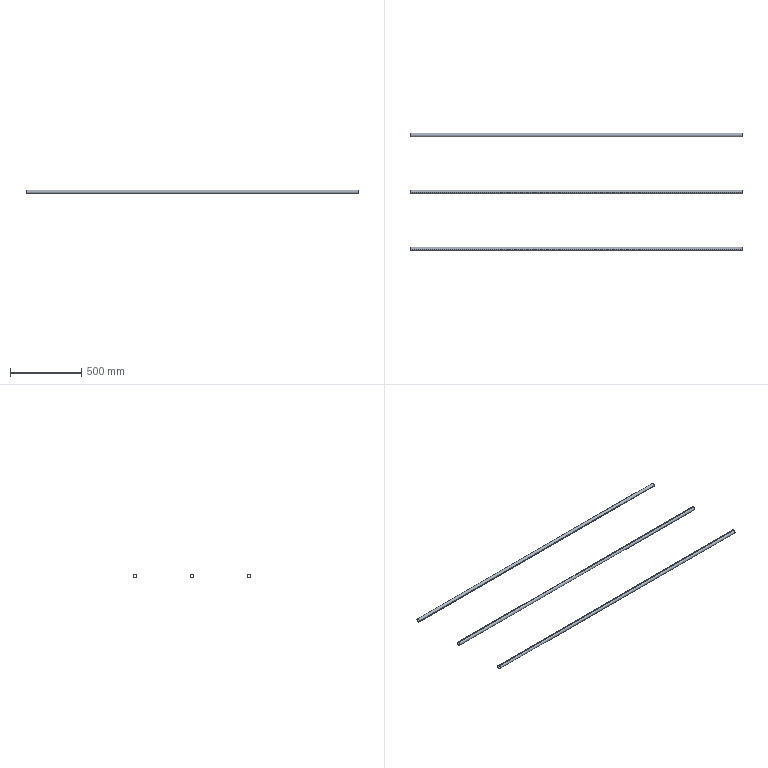Part | STEP file | 粉仓护栏栏杆9_Default<As Machined> | 3 solids | 18 faces | box 2325 x 825 x 25 mm | volume 772419 mm3 | cylinder 12 | plane 6 | commonest cylinder face diameters 22 x6 25 x6
STEP:
#1=CARTESIAN_POINT('',(0.,0.,0.));
#2=DIRECTION('',(0.,0.,1.));
#3=DIRECTION('',(1.,0.,0.));
#4=AXIS2_PLACEMENT_3D('',#1,#2,#3);
#5=CARTESIAN_POINT('',(-2325.,0.,12.5));
#6=VERTEX_POINT('',#5);
#7=CARTESIAN_POINT('',(-2325.,0.,-12.5));
#8=VERTEX_POINT('',#7);
#9=CARTESIAN_POINT('',(-2325.,0.,0.));
#10=DIRECTION('',(-1.,0.,0.));
#11=DIRECTION('',(0.,-1.,0.));
#12=AXIS2_PLACEMENT_3D('',#9,#10,#11);
#13=CIRCLE('',#12,12.5);
#14=CARTESIAN_POINT('',(-2325.,0.,0.));
#15=DIRECTION('',(1.,0.,0.));
#16=DIRECTION('',(0.,0.,-1.));
#17=AXIS2_PLACEMENT_3D('',#14,#15,#16);
#18=CYLINDRICAL_SURFACE('',#17,12.5);
#19=CARTESIAN_POINT('',(4.712,0.));
#20=DIRECTION('',(-1.,0.));
#21=VECTOR('',#20,1.);
#22=LINE('',#19,#21);
#23=(GEOMETRIC_REPRESENTATION_CONTEXT(2)PARAMETRIC_REPRESENTATION_CONTEXT()REPRESENTATION_CONTEXT('',''));
#24=DEFINITIONAL_REPRESENTATION('',(#22),#23);
#25=PCURVE('',#18,#24);
#26=CARTESIAN_POINT('',(-2325.,0.,0.));
#27=DIRECTION('',(-1.,0.,0.));
#28=DIRECTION('',(0.,-1.,0.));
#29=AXIS2_PLACEMENT_3D('',#26,#27,#28);
#30=PLANE('',#29);
#31=CARTESIAN_POINT('',(0.,0.));
#32=DIRECTION('',(1.,0.));
#33=AXIS2_PLACEMENT_2D('',#31,#32);
#34=CIRCLE('',#33,12.5);
#35=(GEOMETRIC_REPRESENTATION_CONTEXT(2)PARAMETRIC_REPRESENTATION_CONTEXT()REPRESENTATION_CONTEXT('',''));
#36=DEFINITIONAL_REPRESENTATION('',(#34),#35);
#37=PCURVE('',#30,#36);
#38=SURFACE_CURVE('',#13,(#25,#37),.PCURVE_S1.);
#39=EDGE_CURVE('',#6,#8,#38,.T.);
#40=ORIENTED_EDGE('',*,*,#39,.F.);
#41=CARTESIAN_POINT('',(0.,0.,12.5));
#42=VERTEX_POINT('',#41);
#43=CARTESIAN_POINT('',(-2325.,0.,12.5));
#44=DIRECTION('',(1.,0.,0.));
#45=VECTOR('',#44,1.);
#46=LINE('',#43,#45);
#47=CARTESIAN_POINT('',(3.142,0.));
#48=DIRECTION('',(0.,1.));
#49=VECTOR('',#48,1.);
#50=LINE('',#47,#49);
#51=(GEOMETRIC_REPRESENTATION_CONTEXT(2)PARAMETRIC_REPRESENTATION_CONTEXT()REPRESENTATION_CONTEXT('',''));
#52=DEFINITIONAL_REPRESENTATION('',(#50),#51);
#53=PCURVE('',#18,#52);
#54=CARTESIAN_POINT('',(-2325.,0.,0.));
#55=DIRECTION('',(1.,0.,0.));
#56=DIRECTION('',(0.,0.,-1.));
#57=AXIS2_PLACEMENT_3D('',#54,#55,#56);
#58=CYLINDRICAL_SURFACE('',#57,12.5);
#59=CARTESIAN_POINT('',(3.142,0.));
#60=DIRECTION('',(0.,1.));
#61=VECTOR('',#60,1.);
#62=LINE('',#59,#61);
#63=(GEOMETRIC_REPRESENTATION_CONTEXT(2)PARAMETRIC_REPRESENTATION_CONTEXT()REPRESENTATION_CONTEXT('',''));
#64=DEFINITIONAL_REPRESENTATION('',(#62),#63);
#65=PCURVE('',#58,#64);
#66=SURFACE_CURVE('',#46,(#53,#65),.PCURVE_S1.);
#67=EDGE_CURVE('',#6,#42,#66,.T.);
#68=ORIENTED_EDGE('',*,*,#67,.T.);
#69=CARTESIAN_POINT('',(0.,0.,-12.5));
#70=VERTEX_POINT('',#69);
#71=CARTESIAN_POINT('',(0.,0.,0.));
#72=DIRECTION('',(-1.,0.,0.));
#73=DIRECTION('',(0.,-1.,0.));
#74=AXIS2_PLACEMENT_3D('',#71,#72,#73);
#75=CIRCLE('',#74,12.5);
#76=CARTESIAN_POINT('',(4.712,2325.));
#77=DIRECTION('',(-1.,0.));
#78=VECTOR('',#77,1.);
#79=LINE('',#76,#78);
#80=(GEOMETRIC_REPRESENTATION_CONTEXT(2)PARAMETRIC_REPRESENTATION_CONTEXT()REPRESENTATION_CONTEXT('',''));
#81=DEFINITIONAL_REPRESENTATION('',(#79),#80);
#82=PCURVE('',#18,#81);
#83=CARTESIAN_POINT('',(0.,0.,0.));
#84=DIRECTION('',(-1.,0.,0.));
#85=DIRECTION('',(0.,-1.,0.));
#86=AXIS2_PLACEMENT_3D('',#83,#84,#85);
#87=PLANE('',#86);
#88=CARTESIAN_POINT('',(0.,0.));
#89=DIRECTION('',(1.,0.));
#90=AXIS2_PLACEMENT_2D('',#88,#89);
#91=CIRCLE('',#90,12.5);
#92=(GEOMETRIC_REPRESENTATION_CONTEXT(2)PARAMETRIC_REPRESENTATION_CONTEXT()REPRESENTATION_CONTEXT('',''));
#93=DEFINITIONAL_REPRESENTATION('',(#91),#92);
#94=PCURVE('',#87,#93);
#95=SURFACE_CURVE('',#75,(#82,#94),.PCURVE_S1.);
#96=EDGE_CURVE('',#42,#70,#95,.T.);
#97=ORIENTED_EDGE('',*,*,#96,.T.);
#98=CARTESIAN_POINT('',(-2325.,0.,-12.5));
#99=DIRECTION('',(1.,0.,0.));
#100=VECTOR('',#99,1.);
#101=LINE('',#98,#100);
#102=CARTESIAN_POINT('',(0.,0.));
#103=DIRECTION('',(0.,1.));
#104=VECTOR('',#103,1.);
#105=LINE('',#102,#104);
#106=(GEOMETRIC_REPRESENTATION_CONTEXT(2)PARAMETRIC_REPRESENTATION_CONTEXT()REPRESENTATION_CONTEXT('',''));
#107=DEFINITIONAL_REPRESENTATION('',(#105),#106);
#108=PCURVE('',#18,#107);
#109=CARTESIAN_POINT('',(6.283,0.));
#110=DIRECTION('',(0.,1.));
#111=VECTOR('',#110,1.);
#112=LINE('',#109,#111);
#113=(GEOMETRIC_REPRESENTATION_CONTEXT(2)PARAMETRIC_REPRESENTATION_CONTEXT()REPRESENTATION_CONTEXT('',''));
#114=DEFINITIONAL_REPRESENTATION('',(#112),#113);
#115=PCURVE('',#58,#114);
#116=SURFACE_CURVE('',#101,(#108,#115),.PCURVE_S1.);
#117=EDGE_CURVE('',#8,#70,#116,.T.);
#118=ORIENTED_EDGE('',*,*,#117,.F.);
#119=EDGE_LOOP('',(#40,#68,#97,#118));
#120=FACE_BOUND('',#119,.T.);
#121=ADVANCED_FACE('',(#120),#18,.T.);
#122=CARTESIAN_POINT('',(-2325.,0.,-11.));
#123=VERTEX_POINT('',#122);
#124=CARTESIAN_POINT('',(0.,0.,-11.));
#125=VERTEX_POINT('',#124);
#126=CARTESIAN_POINT('',(-2325.,0.,-11.));
#127=DIRECTION('',(1.,0.,0.));
#128=VECTOR('',#127,1.);
#129=LINE('',#126,#128);
#130=CARTESIAN_POINT('',(-2325.,0.,0.));
#131=DIRECTION('',(1.,0.,0.));
#132=DIRECTION('',(0.,0.,-1.));
#133=AXIS2_PLACEMENT_3D('',#130,#131,#132);
#134=CYLINDRICAL_SURFACE('',#133,11.);
#135=CARTESIAN_POINT('',(6.283,0.));
#136=DIRECTION('',(0.,1.));
#137=VECTOR('',#136,1.);
#138=LINE('',#135,#137);
#139=(GEOMETRIC_REPRESENTATION_CONTEXT(2)PARAMETRIC_REPRESENTATION_CONTEXT()REPRESENTATION_CONTEXT('',''));
#140=DEFINITIONAL_REPRESENTATION('',(#138),#139);
#141=PCURVE('',#134,#140);
#142=CARTESIAN_POINT('',(-2325.,0.,0.));
#143=DIRECTION('',(1.,0.,0.));
#144=DIRECTION('',(0.,0.,-1.));
#145=AXIS2_PLACEMENT_3D('',#142,#143,#144);
#146=CYLINDRICAL_SURFACE('',#145,11.);
#147=CARTESIAN_POINT('',(0.,0.));
#148=DIRECTION('',(0.,1.));
#149=VECTOR('',#148,1.);
#150=LINE('',#147,#149);
#151=(GEOMETRIC_REPRESENTATION_CONTEXT(2)PARAMETRIC_REPRESENTATION_CONTEXT()REPRESENTATION_CONTEXT('',''));
#152=DEFINITIONAL_REPRESENTATION('',(#150),#151);
#153=PCURVE('',#146,#152);
#154=SURFACE_CURVE('',#129,(#141,#153),.PCURVE_S1.);
#155=EDGE_CURVE('',#123,#125,#154,.T.);
#156=ORIENTED_EDGE('',*,*,#155,.T.);
#157=CARTESIAN_POINT('',(0.,0.,11.));
#158=VERTEX_POINT('',#157);
#159=CARTESIAN_POINT('',(0.,0.,0.));
#160=DIRECTION('',(-1.,0.,0.));
#161=DIRECTION('',(0.,-1.,0.));
#162=AXIS2_PLACEMENT_3D('',#159,#160,#161);
#163=CIRCLE('',#162,11.);
#164=CARTESIAN_POINT('',(10.996,2325.));
#165=DIRECTION('',(-1.,0.));
#166=VECTOR('',#165,1.);
#167=LINE('',#164,#166);
#168=(GEOMETRIC_REPRESENTATION_CONTEXT(2)PARAMETRIC_REPRESENTATION_CONTEXT()REPRESENTATION_CONTEXT('',''));
#169=DEFINITIONAL_REPRESENTATION('',(#167),#168);
#170=PCURVE('',#134,#169);
#171=CARTESIAN_POINT('',(0.,0.));
#172=DIRECTION('',(1.,0.));
#173=AXIS2_PLACEMENT_2D('',#171,#172);
#174=CIRCLE('',#173,11.);
#175=(GEOMETRIC_REPRESENTATION_CONTEXT(2)PARAMETRIC_REPRESENTATION_CONTEXT()REPRESENTATION_CONTEXT('',''));
#176=DEFINITIONAL_REPRESENTATION('',(#174),#175);
#177=PCURVE('',#87,#176);
#178=SURFACE_CURVE('',#163,(#170,#177),.PCURVE_S1.);
#179=EDGE_CURVE('',#125,#158,#178,.T.);
#180=ORIENTED_EDGE('',*,*,#179,.T.);
#181=CARTESIAN_POINT('',(-2325.,0.,11.));
#182=VERTEX_POINT('',#181);
#183=CARTESIAN_POINT('',(-2325.,0.,11.));
#184=DIRECTION('',(1.,0.,0.));
#185=VECTOR('',#184,1.);
#186=LINE('',#183,#185);
#187=CARTESIAN_POINT('',(3.142,0.));
#188=DIRECTION('',(0.,1.));
#189=VECTOR('',#188,1.);
#190=LINE('',#187,#189);
#191=(GEOMETRIC_REPRESENTATION_CONTEXT(2)PARAMETRIC_REPRESENTATION_CONTEXT()REPRESENTATION_CONTEXT('',''));
#192=DEFINITIONAL_REPRESENTATION('',(#190),#191);
#193=PCURVE('',#134,#192);
#194=CARTESIAN_POINT('',(3.142,0.));
#195=DIRECTION('',(0.,1.));
#196=VECTOR('',#195,1.);
#197=LINE('',#194,#196);
#198=(GEOMETRIC_REPRESENTATION_CONTEXT(2)PARAMETRIC_REPRESENTATION_CONTEXT()REPRESENTATION_CONTEXT('',''));
#199=DEFINITIONAL_REPRESENTATION('',(#197),#198);
#200=PCURVE('',#146,#199);
#201=SURFACE_CURVE('',#186,(#193,#200),.PCURVE_S1.);
#202=EDGE_CURVE('',#182,#158,#201,.T.);
#203=ORIENTED_EDGE('',*,*,#202,.F.);
#204=CARTESIAN_POINT('',(-2325.,0.,0.));
#205=DIRECTION('',(-1.,0.,0.));
#206=DIRECTION('',(0.,-1.,0.));
#207=AXIS2_PLACEMENT_3D('',#204,#205,#206);
#208=CIRCLE('',#207,11.);
#209=CARTESIAN_POINT('',(10.996,0.));
#210=DIRECTION('',(-1.,0.));
#211=VECTOR('',#210,1.);
#212=LINE('',#209,#211);
#213=(GEOMETRIC_REPRESENTATION_CONTEXT(2)PARAMETRIC_REPRESENTATION_CONTEXT()REPRESENTATION_CONTEXT('',''));
#214=DEFINITIONAL_REPRESENTATION('',(#212),#213);
#215=PCURVE('',#134,#214);
#216=CARTESIAN_POINT('',(0.,0.));
#217=DIRECTION('',(1.,0.));
#218=AXIS2_PLACEMENT_2D('',#216,#217);
#219=CIRCLE('',#218,11.);
#220=(GEOMETRIC_REPRESENTATION_CONTEXT(2)PARAMETRIC_REPRESENTATION_CONTEXT()REPRESENTATION_CONTEXT('',''));
#221=DEFINITIONAL_REPRESENTATION('',(#219),#220);
#222=PCURVE('',#30,#221);
#223=SURFACE_CURVE('',#208,(#215,#222),.PCURVE_S1.);
#224=EDGE_CURVE('',#123,#182,#223,.T.);
#225=ORIENTED_EDGE('',*,*,#224,.F.);
#226=EDGE_LOOP('',(#156,#180,#203,#225));
#227=FACE_BOUND('',#226,.F.);
#228=ADVANCED_FACE('',(#227),#134,.F.);
#229=CARTESIAN_POINT('',(0.,0.,0.));
#230=DIRECTION('',(-1.,0.,0.));
#231=DIRECTION('',(0.,-1.,0.));
#232=AXIS2_PLACEMENT_3D('',#229,#230,#231);
#233=CIRCLE('',#232,11.);
#234=CARTESIAN_POINT('',(4.712,2325.));
#235=DIRECTION('',(-1.,0.));
#236=VECTOR('',#235,1.);
#237=LINE('',#234,#236);
#238=(GEOMETRIC_REPRESENTATION_CONTEXT(2)PARAMETRIC_REPRESENTATION_CONTEXT()REPRESENTATION_CONTEXT('',''));
#239=DEFINITIONAL_REPRESENTATION('',(#237),#238);
#240=PCURVE('',#146,#239);
#241=CARTESIAN_POINT('',(0.,0.));
#242=DIRECTION('',(1.,0.));
#243=AXIS2_PLACEMENT_2D('',#241,#242);
#244=CIRCLE('',#243,11.);
#245=(GEOMETRIC_REPRESENTATION_CONTEXT(2)PARAMETRIC_REPRESENTATION_CONTEXT()REPRESENTATION_CONTEXT('',''));
#246=DEFINITIONAL_REPRESENTATION('',(#244),#245);
#247=PCURVE('',#87,#246);
#248=SURFACE_CURVE('',#233,(#240,#247),.PCURVE_S1.);
#249=EDGE_CURVE('',#158,#125,#248,.T.);
#250=ORIENTED_EDGE('',*,*,#249,.T.);
#251=ORIENTED_EDGE('',*,*,#155,.F.);
#252=CARTESIAN_POINT('',(-2325.,0.,0.));
#253=DIRECTION('',(-1.,0.,0.));
#254=DIRECTION('',(0.,-1.,0.));
#255=AXIS2_PLACEMENT_3D('',#252,#253,#254);
#256=CIRCLE('',#255,11.);
#257=CARTESIAN_POINT('',(4.712,0.));
#258=DIRECTION('',(-1.,0.));
#259=VECTOR('',#258,1.);
#260=LINE('',#257,#259);
#261=(GEOMETRIC_REPRESENTATION_CONTEXT(2)PARAMETRIC_REPRESENTATION_CONTEXT()REPRESENTATION_CONTEXT('',''));
#262=DEFINITIONAL_REPRESENTATION('',(#260),#261);
#263=PCURVE('',#146,#262);
#264=CARTESIAN_POINT('',(0.,0.));
#265=DIRECTION('',(1.,0.));
#266=AXIS2_PLACEMENT_2D('',#264,#265);
#267=CIRCLE('',#266,11.);
#268=(GEOMETRIC_REPRESENTATION_CONTEXT(2)PARAMETRIC_REPRESENTATION_CONTEXT()REPRESENTATION_CONTEXT('',''));
#269=DEFINITIONAL_REPRESENTATION('',(#267),#268);
#270=PCURVE('',#30,#269);
#271=SURFACE_CURVE('',#256,(#263,#270),.PCURVE_S1.);
#272=EDGE_CURVE('',#182,#123,#271,.T.);
#273=ORIENTED_EDGE('',*,*,#272,.F.);
#274=ORIENTED_EDGE('',*,*,#202,.T.);
#275=EDGE_LOOP('',(#250,#251,#273,#274));
#276=FACE_BOUND('',#275,.F.);
#277=ADVANCED_FACE('',(#276),#146,.F.);
#278=ORIENTED_EDGE('',*,*,#67,.F.);
#279=CARTESIAN_POINT('',(-2325.,0.,0.));
#280=DIRECTION('',(-1.,0.,0.));
#281=DIRECTION('',(0.,-1.,0.));
#282=AXIS2_PLACEMENT_3D('',#279,#280,#281);
#283=CIRCLE('',#282,12.5);
#284=CARTESIAN_POINT('',(10.996,0.));
#285=DIRECTION('',(-1.,0.));
#286=VECTOR('',#285,1.);
#287=LINE('',#284,#286);
#288=(GEOMETRIC_REPRESENTATION_CONTEXT(2)PARAMETRIC_REPRESENTATION_CONTEXT()REPRESENTATION_CONTEXT('',''));
#289=DEFINITIONAL_REPRESENTATION('',(#287),#288);
#290=PCURVE('',#58,#289);
#291=CARTESIAN_POINT('',(0.,0.));
#292=DIRECTION('',(1.,0.));
#293=AXIS2_PLACEMENT_2D('',#291,#292);
#294=CIRCLE('',#293,12.5);
#295=(GEOMETRIC_REPRESENTATION_CONTEXT(2)PARAMETRIC_REPRESENTATION_CONTEXT()REPRESENTATION_CONTEXT('',''));
#296=DEFINITIONAL_REPRESENTATION('',(#294),#295);
#297=PCURVE('',#30,#296);
#298=SURFACE_CURVE('',#283,(#290,#297),.PCURVE_S1.);
#299=EDGE_CURVE('',#8,#6,#298,.T.);
#300=ORIENTED_EDGE('',*,*,#299,.F.);
#301=ORIENTED_EDGE('',*,*,#117,.T.);
#302=CARTESIAN_POINT('',(0.,0.,0.));
#303=DIRECTION('',(-1.,0.,0.));
#304=DIRECTION('',(0.,-1.,0.));
#305=AXIS2_PLACEMENT_3D('',#302,#303,#304);
#306=CIRCLE('',#305,12.5);
#307=CARTESIAN_POINT('',(10.996,2325.));
#308=DIRECTION('',(-1.,0.));
#309=VECTOR('',#308,1.);
#310=LINE('',#307,#309);
#311=(GEOMETRIC_REPRESENTATION_CONTEXT(2)PARAMETRIC_REPRESENTATION_CONTEXT()REPRESENTATION_CONTEXT('',''));
#312=DEFINITIONAL_REPRESENTATION('',(#310),#311);
#313=PCURVE('',#58,#312);
#314=CARTESIAN_POINT('',(0.,0.));
#315=DIRECTION('',(1.,0.));
#316=AXIS2_PLACEMENT_2D('',#314,#315);
#317=CIRCLE('',#316,12.5);
#318=(GEOMETRIC_REPRESENTATION_CONTEXT(2)PARAMETRIC_REPRESENTATION_CONTEXT()REPRESENTATION_CONTEXT('',''));
#319=DEFINITIONAL_REPRESENTATION('',(#317),#318);
#320=PCURVE('',#87,#319);
#321=SURFACE_CURVE('',#306,(#313,#320),.PCURVE_S1.);
#322=EDGE_CURVE('',#70,#42,#321,.T.);
#323=ORIENTED_EDGE('',*,*,#322,.T.);
#324=EDGE_LOOP('',(#278,#300,#301,#323));
#325=FACE_BOUND('',#324,.T.);
#326=ADVANCED_FACE('',(#325),#58,.T.);
#327=ORIENTED_EDGE('',*,*,#224,.F.);
#328=ORIENTED_EDGE('',*,*,#272,.F.);
#329=EDGE_LOOP('',(#327,#328));
#330=FACE_BOUND('',#329,.T.);
#331=ORIENTED_EDGE('',*,*,#299,.T.);
#332=ORIENTED_EDGE('',*,*,#39,.T.);
#333=EDGE_LOOP('',(#331,#332));
#334=FACE_BOUND('',#333,.T.);
#335=ADVANCED_FACE('',(#330,#334),#30,.T.);
#336=ORIENTED_EDGE('',*,*,#179,.T.);
#337=ORIENTED_EDGE('',*,*,#249,.T.);
#338=EDGE_LOOP('',(#336,#337));
#339=FACE_BOUND('',#338,.T.);
#340=ORIENTED_EDGE('',*,*,#322,.F.);
#341=ORIENTED_EDGE('',*,*,#96,.F.);
#342=EDGE_LOOP('',(#340,#341));
#343=FACE_BOUND('',#342,.T.);
#344=ADVANCED_FACE('',(#339,#343),#87,.F.);
#345=CLOSED_SHELL('',(#121,#228,#277,#326,#335,#344));
#346=MANIFOLD_SOLID_BREP('',#345);
#347=CARTESIAN_POINT('',(-2325.,787.5,0.));
#348=VERTEX_POINT('',#347);
#349=CARTESIAN_POINT('',(-2325.,812.5,0.));
#350=VERTEX_POINT('',#349);
#351=CARTESIAN_POINT('',(-2325.,800.,0.));
#352=DIRECTION('',(-1.,0.,0.));
#353=DIRECTION('',(0.,-1.,0.));
#354=AXIS2_PLACEMENT_3D('',#351,#352,#353);
#355=CIRCLE('',#354,12.5);
#356=CARTESIAN_POINT('',(-2325.,800.,0.));
#357=DIRECTION('',(1.,0.,0.));
#358=DIRECTION('',(0.,1.,0.));
#359=AXIS2_PLACEMENT_3D('',#356,#357,#358);
#360=CYLINDRICAL_SURFACE('',#359,12.5);
#361=CARTESIAN_POINT('',(3.142,0.));
#362=DIRECTION('',(-1.,0.));
#363=VECTOR('',#362,1.);
#364=LINE('',#361,#363);
#365=(GEOMETRIC_REPRESENTATION_CONTEXT(2)PARAMETRIC_REPRESENTATION_CONTEXT()REPRESENTATION_CONTEXT('',''));
#366=DEFINITIONAL_REPRESENTATION('',(#364),#365);
#367=PCURVE('',#360,#366);
#368=CARTESIAN_POINT('',(-2325.,800.,0.));
#369=DIRECTION('',(-1.,0.,0.));
#370=DIRECTION('',(0.,-1.,0.));
#371=AXIS2_PLACEMENT_3D('',#368,#369,#370);
#372=PLANE('',#371);
#373=CARTESIAN_POINT('',(0.,0.));
#374=DIRECTION('',(1.,0.));
#375=AXIS2_PLACEMENT_2D('',#373,#374);
#376=CIRCLE('',#375,12.5);
#377=(GEOMETRIC_REPRESENTATION_CONTEXT(2)PARAMETRIC_REPRESENTATION_CONTEXT()REPRESENTATION_CONTEXT('',''));
#378=DEFINITIONAL_REPRESENTATION('',(#376),#377);
#379=PCURVE('',#372,#378);
#380=SURFACE_CURVE('',#355,(#367,#379),.PCURVE_S1.);
#381=EDGE_CURVE('',#348,#350,#380,.T.);
#382=ORIENTED_EDGE('',*,*,#381,.F.);
#383=CARTESIAN_POINT('',(0.,787.5,0.));
#384=VERTEX_POINT('',#383);
#385=CARTESIAN_POINT('',(-2325.,787.5,0.));
#386=DIRECTION('',(1.,0.,0.));
#387=VECTOR('',#386,1.);
#388=LINE('',#385,#387);
#389=CARTESIAN_POINT('',(3.142,0.));
#390=DIRECTION('',(0.,1.));
#391=VECTOR('',#390,1.);
#392=LINE('',#389,#391);
#393=(GEOMETRIC_REPRESENTATION_CONTEXT(2)PARAMETRIC_REPRESENTATION_CONTEXT()REPRESENTATION_CONTEXT('',''));
#394=DEFINITIONAL_REPRESENTATION('',(#392),#393);
#395=PCURVE('',#360,#394);
#396=CARTESIAN_POINT('',(-2325.,800.,0.));
#397=DIRECTION('',(1.,0.,0.));
#398=DIRECTION('',(0.,1.,0.));
#399=AXIS2_PLACEMENT_3D('',#396,#397,#398);
#400=CYLINDRICAL_SURFACE('',#399,12.5);
#401=CARTESIAN_POINT('',(3.142,0.));
#402=DIRECTION('',(0.,1.));
#403=VECTOR('',#402,1.);
#404=LINE('',#401,#403);
#405=(GEOMETRIC_REPRESENTATION_CONTEXT(2)PARAMETRIC_REPRESENTATION_CONTEXT()REPRESENTATION_CONTEXT('',''));
#406=DEFINITIONAL_REPRESENTATION('',(#404),#405);
#407=PCURVE('',#400,#406);
#408=SURFACE_CURVE('',#388,(#395,#407),.PCURVE_S1.);
#409=EDGE_CURVE('',#348,#384,#408,.T.);
#410=ORIENTED_EDGE('',*,*,#409,.T.);
#411=CARTESIAN_POINT('',(0.,812.5,0.));
#412=VERTEX_POINT('',#411);
#413=CARTESIAN_POINT('',(0.,800.,0.));
#414=DIRECTION('',(-1.,0.,0.));
#415=DIRECTION('',(0.,-1.,0.));
#416=AXIS2_PLACEMENT_3D('',#413,#414,#415);
#417=CIRCLE('',#416,12.5);
#418=CARTESIAN_POINT('',(3.142,2325.));
#419=DIRECTION('',(-1.,0.));
#420=VECTOR('',#419,1.);
#421=LINE('',#418,#420);
#422=(GEOMETRIC_REPRESENTATION_CONTEXT(2)PARAMETRIC_REPRESENTATION_CONTEXT()REPRESENTATION_CONTEXT('',''));
#423=DEFINITIONAL_REPRESENTATION('',(#421),#422);
#424=PCURVE('',#360,#423);
#425=CARTESIAN_POINT('',(0.,800.,0.));
#426=DIRECTION('',(-1.,0.,0.));
#427=DIRECTION('',(0.,-1.,0.));
#428=AXIS2_PLACEMENT_3D('',#425,#426,#427);
#429=PLANE('',#428);
#430=CARTESIAN_POINT('',(0.,0.));
#431=DIRECTION('',(1.,0.));
#432=AXIS2_PLACEMENT_2D('',#430,#431);
#433=CIRCLE('',#432,12.5);
#434=(GEOMETRIC_REPRESENTATION_CONTEXT(2)PARAMETRIC_REPRESENTATION_CONTEXT()REPRESENTATION_CONTEXT('',''));
#435=DEFINITIONAL_REPRESENTATION('',(#433),#434);
#436=PCURVE('',#429,#435);
#437=SURFACE_CURVE('',#417,(#424,#436),.PCURVE_S1.);
#438=EDGE_CURVE('',#384,#412,#437,.T.);
#439=ORIENTED_EDGE('',*,*,#438,.T.);
#440=CARTESIAN_POINT('',(-2325.,812.5,0.));
#441=DIRECTION('',(1.,0.,0.));
#442=VECTOR('',#441,1.);
#443=LINE('',#440,#442);
#444=CARTESIAN_POINT('',(0.,0.));
#445=DIRECTION('',(0.,1.));
#446=VECTOR('',#445,1.);
#447=LINE('',#444,#446);
#448=(GEOMETRIC_REPRESENTATION_CONTEXT(2)PARAMETRIC_REPRESENTATION_CONTEXT()REPRESENTATION_CONTEXT('',''));
#449=DEFINITIONAL_REPRESENTATION('',(#447),#448);
#450=PCURVE('',#360,#449);
#451=CARTESIAN_POINT('',(6.283,0.));
#452=DIRECTION('',(0.,1.));
#453=VECTOR('',#452,1.);
#454=LINE('',#451,#453);
#455=(GEOMETRIC_REPRESENTATION_CONTEXT(2)PARAMETRIC_REPRESENTATION_CONTEXT()REPRESENTATION_CONTEXT('',''));
#456=DEFINITIONAL_REPRESENTATION('',(#454),#455);
#457=PCURVE('',#400,#456);
#458=SURFACE_CURVE('',#443,(#450,#457),.PCURVE_S1.);
#459=EDGE_CURVE('',#350,#412,#458,.T.);
#460=ORIENTED_EDGE('',*,*,#459,.F.);
#461=EDGE_LOOP('',(#382,#410,#439,#460));
#462=FACE_BOUND('',#461,.T.);
#463=ADVANCED_FACE('',(#462),#360,.T.);
#464=CARTESIAN_POINT('',(-2325.,811.,0.));
#465=VERTEX_POINT('',#464);
#466=CARTESIAN_POINT('',(0.,811.,0.));
#467=VERTEX_POINT('',#466);
#468=CARTESIAN_POINT('',(-2325.,811.,0.));
#469=DIRECTION('',(1.,0.,0.));
#470=VECTOR('',#469,1.);
#471=LINE('',#468,#470);
#472=CARTESIAN_POINT('',(-2325.,800.,0.));
#473=DIRECTION('',(1.,0.,0.));
#474=DIRECTION('',(0.,1.,0.));
#475=AXIS2_PLACEMENT_3D('',#472,#473,#474);
#476=CYLINDRICAL_SURFACE('',#475,11.);
#477=CARTESIAN_POINT('',(6.283,0.));
#478=DIRECTION('',(0.,1.));
#479=VECTOR('',#478,1.);
#480=LINE('',#477,#479);
#481=(GEOMETRIC_REPRESENTATION_CONTEXT(2)PARAMETRIC_REPRESENTATION_CONTEXT()REPRESENTATION_CONTEXT('',''));
#482=DEFINITIONAL_REPRESENTATION('',(#480),#481);
#483=PCURVE('',#476,#482);
#484=CARTESIAN_POINT('',(-2325.,800.,0.));
#485=DIRECTION('',(1.,0.,0.));
#486=DIRECTION('',(0.,1.,0.));
#487=AXIS2_PLACEMENT_3D('',#484,#485,#486);
#488=CYLINDRICAL_SURFACE('',#487,11.);
#489=CARTESIAN_POINT('',(0.,0.));
#490=DIRECTION('',(0.,1.));
#491=VECTOR('',#490,1.);
#492=LINE('',#489,#491);
#493=(GEOMETRIC_REPRESENTATION_CONTEXT(2)PARAMETRIC_REPRESENTATION_CONTEXT()REPRESENTATION_CONTEXT('',''));
#494=DEFINITIONAL_REPRESENTATION('',(#492),#493);
#495=PCURVE('',#488,#494);
#496=SURFACE_CURVE('',#471,(#483,#495),.PCURVE_S1.);
#497=EDGE_CURVE('',#465,#467,#496,.T.);
#498=ORIENTED_EDGE('',*,*,#497,.T.);
#499=CARTESIAN_POINT('',(0.,789.,0.));
#500=VERTEX_POINT('',#499);
#501=CARTESIAN_POINT('',(0.,800.,0.));
#502=DIRECTION('',(-1.,0.,0.));
#503=DIRECTION('',(0.,-1.,0.));
#504=AXIS2_PLACEMENT_3D('',#501,#502,#503);
#505=CIRCLE('',#504,11.);
#506=CARTESIAN_POINT('',(9.425,2325.));
#507=DIRECTION('',(-1.,0.));
#508=VECTOR('',#507,1.);
#509=LINE('',#506,#508);
#510=(GEOMETRIC_REPRESENTATION_CONTEXT(2)PARAMETRIC_REPRESENTATION_CONTEXT()REPRESENTATION_CONTEXT('',''));
#511=DEFINITIONAL_REPRESENTATION('',(#509),#510);
#512=PCURVE('',#476,#511);
#513=CARTESIAN_POINT('',(0.,0.));
#514=DIRECTION('',(1.,0.));
#515=AXIS2_PLACEMENT_2D('',#513,#514);
#516=CIRCLE('',#515,11.);
#517=(GEOMETRIC_REPRESENTATION_CONTEXT(2)PARAMETRIC_REPRESENTATION_CONTEXT()REPRESENTATION_CONTEXT('',''));
#518=DEFINITIONAL_REPRESENTATION('',(#516),#517);
#519=PCURVE('',#429,#518);
#520=SURFACE_CURVE('',#505,(#512,#519),.PCURVE_S1.);
#521=EDGE_CURVE('',#467,#500,#520,.T.);
#522=ORIENTED_EDGE('',*,*,#521,.T.);
#523=CARTESIAN_POINT('',(-2325.,789.,0.));
#524=VERTEX_POINT('',#523);
#525=CARTESIAN_POINT('',(-2325.,789.,0.));
#526=DIRECTION('',(1.,0.,0.));
#527=VECTOR('',#526,1.);
#528=LINE('',#525,#527);
#529=CARTESIAN_POINT('',(3.142,0.));
#530=DIRECTION('',(0.,1.));
#531=VECTOR('',#530,1.);
#532=LINE('',#529,#531);
#533=(GEOMETRIC_REPRESENTATION_CONTEXT(2)PARAMETRIC_REPRESENTATION_CONTEXT()REPRESENTATION_CONTEXT('',''));
#534=DEFINITIONAL_REPRESENTATION('',(#532),#533);
#535=PCURVE('',#476,#534);
#536=CARTESIAN_POINT('',(3.142,0.));
#537=DIRECTION('',(0.,1.));
#538=VECTOR('',#537,1.);
#539=LINE('',#536,#538);
#540=(GEOMETRIC_REPRESENTATION_CONTEXT(2)PARAMETRIC_REPRESENTATION_CONTEXT()REPRESENTATION_CONTEXT('',''));
#541=DEFINITIONAL_REPRESENTATION('',(#539),#540);
#542=PCURVE('',#488,#541);
#543=SURFACE_CURVE('',#528,(#535,#542),.PCURVE_S1.);
#544=EDGE_CURVE('',#524,#500,#543,.T.);
#545=ORIENTED_EDGE('',*,*,#544,.F.);
#546=CARTESIAN_POINT('',(-2325.,800.,0.));
#547=DIRECTION('',(-1.,0.,0.));
#548=DIRECTION('',(0.,-1.,0.));
#549=AXIS2_PLACEMENT_3D('',#546,#547,#548);
#550=CIRCLE('',#549,11.);
#551=CARTESIAN_POINT('',(9.425,0.));
#552=DIRECTION('',(-1.,0.));
#553=VECTOR('',#552,1.);
#554=LINE('',#551,#553);
#555=(GEOMETRIC_REPRESENTATION_CONTEXT(2)PARAMETRIC_REPRESENTATION_CONTEXT()REPRESENTATION_CONTEXT('',''));
#556=DEFINITIONAL_REPRESENTATION('',(#554),#555);
#557=PCURVE('',#476,#556);
#558=CARTESIAN_POINT('',(0.,0.));
#559=DIRECTION('',(1.,0.));
#560=AXIS2_PLACEMENT_2D('',#558,#559);
#561=CIRCLE('',#560,11.);
#562=(GEOMETRIC_REPRESENTATION_CONTEXT(2)PARAMETRIC_REPRESENTATION_CONTEXT()REPRESENTATION_CONTEXT('',''));
#563=DEFINITIONAL_REPRESENTATION('',(#561),#562);
#564=PCURVE('',#372,#563);
#565=SURFACE_CURVE('',#550,(#557,#564),.PCURVE_S1.);
#566=EDGE_CURVE('',#465,#524,#565,.T.);
#567=ORIENTED_EDGE('',*,*,#566,.F.);
#568=EDGE_LOOP('',(#498,#522,#545,#567));
#569=FACE_BOUND('',#568,.F.);
#570=ADVANCED_FACE('',(#569),#476,.F.);
#571=CARTESIAN_POINT('',(0.,800.,0.));
#572=DIRECTION('',(-1.,0.,0.));
#573=DIRECTION('',(0.,-1.,0.));
#574=AXIS2_PLACEMENT_3D('',#571,#572,#573);
#575=CIRCLE('',#574,11.);
#576=CARTESIAN_POINT('',(3.142,2325.));
#577=DIRECTION('',(-1.,0.));
#578=VECTOR('',#577,1.);
#579=LINE('',#576,#578);
#580=(GEOMETRIC_REPRESENTATION_CONTEXT(2)PARAMETRIC_REPRESENTATION_CONTEXT()REPRESENTATION_CONTEXT('',''));
#581=DEFINITIONAL_REPRESENTATION('',(#579),#580);
#582=PCURVE('',#488,#581);
#583=CARTESIAN_POINT('',(0.,0.));
#584=DIRECTION('',(1.,0.));
#585=AXIS2_PLACEMENT_2D('',#583,#584);
#586=CIRCLE('',#585,11.);
#587=(GEOMETRIC_REPRESENTATION_CONTEXT(2)PARAMETRIC_REPRESENTATION_CONTEXT()REPRESENTATION_CONTEXT('',''));
#588=DEFINITIONAL_REPRESENTATION('',(#586),#587);
#589=PCURVE('',#429,#588);
#590=SURFACE_CURVE('',#575,(#582,#589),.PCURVE_S1.);
#591=EDGE_CURVE('',#500,#467,#590,.T.);
#592=ORIENTED_EDGE('',*,*,#591,.T.);
#593=ORIENTED_EDGE('',*,*,#497,.F.);
#594=CARTESIAN_POINT('',(-2325.,800.,0.));
#595=DIRECTION('',(-1.,0.,0.));
#596=DIRECTION('',(0.,-1.,0.));
#597=AXIS2_PLACEMENT_3D('',#594,#595,#596);
#598=CIRCLE('',#597,11.);
#599=CARTESIAN_POINT('',(3.142,0.));
#600=DIRECTION('',(-1.,0.));
#601=VECTOR('',#600,1.);
#602=LINE('',#599,#601);
#603=(GEOMETRIC_REPRESENTATION_CONTEXT(2)PARAMETRIC_REPRESENTATION_CONTEXT()REPRESENTATION_CONTEXT('',''));
#604=DEFINITIONAL_REPRESENTATION('',(#602),#603);
#605=PCURVE('',#488,#604);
#606=CARTESIAN_POINT('',(0.,0.));
#607=DIRECTION('',(1.,0.));
#608=AXIS2_PLACEMENT_2D('',#606,#607);
#609=CIRCLE('',#608,11.);
#610=(GEOMETRIC_REPRESENTATION_CONTEXT(2)PARAMETRIC_REPRESENTATION_CONTEXT()REPRESENTATION_CONTEXT('',''));
#611=DEFINITIONAL_REPRESENTATION('',(#609),#610);
#612=PCURVE('',#372,#611);
#613=SURFACE_CURVE('',#598,(#605,#612),.PCURVE_S1.);
#614=EDGE_CURVE('',#524,#465,#613,.T.);
#615=ORIENTED_EDGE('',*,*,#614,.F.);
#616=ORIENTED_EDGE('',*,*,#544,.T.);
#617=EDGE_LOOP('',(#592,#593,#615,#616));
#618=FACE_BOUND('',#617,.F.);
#619=ADVANCED_FACE('',(#618),#488,.F.);
#620=ORIENTED_EDGE('',*,*,#409,.F.);
#621=CARTESIAN_POINT('',(-2325.,800.,0.));
#622=DIRECTION('',(-1.,0.,0.));
#623=DIRECTION('',(0.,-1.,0.));
#624=AXIS2_PLACEMENT_3D('',#621,#622,#623);
#625=CIRCLE('',#624,12.5);
#626=CARTESIAN_POINT('',(9.425,0.));
#627=DIRECTION('',(-1.,0.));
#628=VECTOR('',#627,1.);
#629=LINE('',#626,#628);
#630=(GEOMETRIC_REPRESENTATION_CONTEXT(2)PARAMETRIC_REPRESENTATION_CONTEXT()REPRESENTATION_CONTEXT('',''));
#631=DEFINITIONAL_REPRESENTATION('',(#629),#630);
#632=PCURVE('',#400,#631);
#633=CARTESIAN_POINT('',(0.,0.));
#634=DIRECTION('',(1.,0.));
#635=AXIS2_PLACEMENT_2D('',#633,#634);
#636=CIRCLE('',#635,12.5);
#637=(GEOMETRIC_REPRESENTATION_CONTEXT(2)PARAMETRIC_REPRESENTATION_CONTEXT()REPRESENTATION_CONTEXT('',''));
#638=DEFINITIONAL_REPRESENTATION('',(#636),#637);
#639=PCURVE('',#372,#638);
#640=SURFACE_CURVE('',#625,(#632,#639),.PCURVE_S1.);
#641=EDGE_CURVE('',#350,#348,#640,.T.);
#642=ORIENTED_EDGE('',*,*,#641,.F.);
#643=ORIENTED_EDGE('',*,*,#459,.T.);
#644=CARTESIAN_POINT('',(0.,800.,0.));
#645=DIRECTION('',(-1.,0.,0.));
#646=DIRECTION('',(0.,-1.,0.));
#647=AXIS2_PLACEMENT_3D('',#644,#645,#646);
#648=CIRCLE('',#647,12.5);
#649=CARTESIAN_POINT('',(9.425,2325.));
#650=DIRECTION('',(-1.,0.));
#651=VECTOR('',#650,1.);
#652=LINE('',#649,#651);
#653=(GEOMETRIC_REPRESENTATION_CONTEXT(2)PARAMETRIC_REPRESENTATION_CONTEXT()REPRESENTATION_CONTEXT('',''));
#654=DEFINITIONAL_REPRESENTATION('',(#652),#653);
#655=PCURVE('',#400,#654);
#656=CARTESIAN_POINT('',(0.,0.));
#657=DIRECTION('',(1.,0.));
#658=AXIS2_PLACEMENT_2D('',#656,#657);
#659=CIRCLE('',#658,12.5);
#660=(GEOMETRIC_REPRESENTATION_CONTEXT(2)PARAMETRIC_REPRESENTATION_CONTEXT()REPRESENTATION_CONTEXT('',''));
#661=DEFINITIONAL_REPRESENTATION('',(#659),#660);
#662=PCURVE('',#429,#661);
#663=SURFACE_CURVE('',#648,(#655,#662),.PCURVE_S1.);
#664=EDGE_CURVE('',#412,#384,#663,.T.);
#665=ORIENTED_EDGE('',*,*,#664,.T.);
#666=EDGE_LOOP('',(#620,#642,#643,#665));
#667=FACE_BOUND('',#666,.T.);
#668=ADVANCED_FACE('',(#667),#400,.T.);
#669=ORIENTED_EDGE('',*,*,#566,.F.);
#670=ORIENTED_EDGE('',*,*,#614,.F.);
#671=EDGE_LOOP('',(#669,#670));
#672=FACE_BOUND('',#671,.T.);
#673=ORIENTED_EDGE('',*,*,#641,.T.);
#674=ORIENTED_EDGE('',*,*,#381,.T.);
#675=EDGE_LOOP('',(#673,#674));
#676=FACE_BOUND('',#675,.T.);
#677=ADVANCED_FACE('',(#672,#676),#372,.T.);
#678=ORIENTED_EDGE('',*,*,#521,.T.);
#679=ORIENTED_EDGE('',*,*,#591,.T.);
#680=EDGE_LOOP('',(#678,#679));
#681=FACE_BOUND('',#680,.T.);
#682=ORIENTED_EDGE('',*,*,#664,.F.);
#683=ORIENTED_EDGE('',*,*,#438,.F.);
#684=EDGE_LOOP('',(#682,#683));
#685=FACE_BOUND('',#684,.T.);
#686=ADVANCED_FACE('',(#681,#685),#429,.F.);
#687=CLOSED_SHELL('',(#463,#570,#619,#668,#677,#686));
#688=MANIFOLD_SOLID_BREP('',#687);
#689=CARTESIAN_POINT('',(0.,400.,-12.5));
#690=VERTEX_POINT('',#689);
#691=CARTESIAN_POINT('',(0.,400.,12.5));
#692=VERTEX_POINT('',#691);
#693=CARTESIAN_POINT('',(0.,400.,0.));
#694=DIRECTION('',(1.,0.,0.));
#695=DIRECTION('',(0.,1.,0.));
#696=AXIS2_PLACEMENT_3D('',#693,#694,#695);
#697=CIRCLE('',#696,12.5);
#698=CARTESIAN_POINT('',(0.,400.,0.));
#699=DIRECTION('',(-1.,0.,0.));
#700=DIRECTION('',(0.,0.,1.));
#701=AXIS2_PLACEMENT_3D('',#698,#699,#700);
#702=CYLINDRICAL_SURFACE('',#701,12.5);
#703=CARTESIAN_POINT('',(7.854,0.));
#704=DIRECTION('',(-1.,0.));
#705=VECTOR('',#704,1.);
#706=LINE('',#703,#705);
#707=(GEOMETRIC_REPRESENTATION_CONTEXT(2)PARAMETRIC_REPRESENTATION_CONTEXT()REPRESENTATION_CONTEXT('',''));
#708=DEFINITIONAL_REPRESENTATION('',(#706),#707);
#709=PCURVE('',#702,#708);
#710=CARTESIAN_POINT('',(0.,400.,0.));
#711=DIRECTION('',(1.,0.,0.));
#712=DIRECTION('',(0.,1.,0.));
#713=AXIS2_PLACEMENT_3D('',#710,#711,#712);
#714=PLANE('',#713);
#715=CARTESIAN_POINT('',(0.,0.));
#716=DIRECTION('',(1.,0.));
#717=AXIS2_PLACEMENT_2D('',#715,#716);
#718=CIRCLE('',#717,12.5);
#719=(GEOMETRIC_REPRESENTATION_CONTEXT(2)PARAMETRIC_REPRESENTATION_CONTEXT()REPRESENTATION_CONTEXT('',''));
#720=DEFINITIONAL_REPRESENTATION('',(#718),#719);
#721=PCURVE('',#714,#720);
#722=SURFACE_CURVE('',#697,(#709,#721),.PCURVE_S1.);
#723=EDGE_CURVE('',#690,#692,#722,.T.);
#724=ORIENTED_EDGE('',*,*,#723,.F.);
#725=CARTESIAN_POINT('',(-2325.,400.,-12.5));
#726=VERTEX_POINT('',#725);
#727=CARTESIAN_POINT('',(0.,400.,-12.5));
#728=DIRECTION('',(-1.,0.,0.));
#729=VECTOR('',#728,1.);
#730=LINE('',#727,#729);
#731=CARTESIAN_POINT('',(3.142,0.));
#732=DIRECTION('',(0.,1.));
#733=VECTOR('',#732,1.);
#734=LINE('',#731,#733);
#735=(GEOMETRIC_REPRESENTATION_CONTEXT(2)PARAMETRIC_REPRESENTATION_CONTEXT()REPRESENTATION_CONTEXT('',''));
#736=DEFINITIONAL_REPRESENTATION('',(#734),#735);
#737=PCURVE('',#702,#736);
#738=CARTESIAN_POINT('',(0.,400.,0.));
#739=DIRECTION('',(-1.,0.,0.));
#740=DIRECTION('',(0.,0.,1.));
#741=AXIS2_PLACEMENT_3D('',#738,#739,#740);
#742=CYLINDRICAL_SURFACE('',#741,12.5);
#743=CARTESIAN_POINT('',(3.142,0.));
#744=DIRECTION('',(0.,1.));
#745=VECTOR('',#744,1.);
#746=LINE('',#743,#745);
#747=(GEOMETRIC_REPRESENTATION_CONTEXT(2)PARAMETRIC_REPRESENTATION_CONTEXT()REPRESENTATION_CONTEXT('',''));
#748=DEFINITIONAL_REPRESENTATION('',(#746),#747);
#749=PCURVE('',#742,#748);
#750=SURFACE_CURVE('',#730,(#737,#749),.PCURVE_S1.);
#751=EDGE_CURVE('',#690,#726,#750,.T.);
#752=ORIENTED_EDGE('',*,*,#751,.T.);
#753=CARTESIAN_POINT('',(-2325.,400.,12.5));
#754=VERTEX_POINT('',#753);
#755=CARTESIAN_POINT('',(-2325.,400.,0.));
#756=DIRECTION('',(1.,0.,0.));
#757=DIRECTION('',(0.,1.,0.));
#758=AXIS2_PLACEMENT_3D('',#755,#756,#757);
#759=CIRCLE('',#758,12.5);
#760=CARTESIAN_POINT('',(7.854,2325.));
#761=DIRECTION('',(-1.,0.));
#762=VECTOR('',#761,1.);
#763=LINE('',#760,#762);
#764=(GEOMETRIC_REPRESENTATION_CONTEXT(2)PARAMETRIC_REPRESENTATION_CONTEXT()REPRESENTATION_CONTEXT('',''));
#765=DEFINITIONAL_REPRESENTATION('',(#763),#764);
#766=PCURVE('',#702,#765);
#767=CARTESIAN_POINT('',(-2325.,400.,0.));
#768=DIRECTION('',(1.,0.,0.));
#769=DIRECTION('',(0.,1.,0.));
#770=AXIS2_PLACEMENT_3D('',#767,#768,#769);
#771=PLANE('',#770);
#772=CARTESIAN_POINT('',(0.,0.));
#773=DIRECTION('',(1.,0.));
#774=AXIS2_PLACEMENT_2D('',#772,#773);
#775=CIRCLE('',#774,12.5);
#776=(GEOMETRIC_REPRESENTATION_CONTEXT(2)PARAMETRIC_REPRESENTATION_CONTEXT()REPRESENTATION_CONTEXT('',''));
#777=DEFINITIONAL_REPRESENTATION('',(#775),#776);
#778=PCURVE('',#771,#777);
#779=SURFACE_CURVE('',#759,(#766,#778),.PCURVE_S1.);
#780=EDGE_CURVE('',#726,#754,#779,.T.);
#781=ORIENTED_EDGE('',*,*,#780,.T.);
#782=CARTESIAN_POINT('',(0.,400.,12.5));
#783=DIRECTION('',(-1.,0.,0.));
#784=VECTOR('',#783,1.);
#785=LINE('',#782,#784);
#786=CARTESIAN_POINT('',(0.,0.));
#787=DIRECTION('',(0.,1.));
#788=VECTOR('',#787,1.);
#789=LINE('',#786,#788);
#790=(GEOMETRIC_REPRESENTATION_CONTEXT(2)PARAMETRIC_REPRESENTATION_CONTEXT()REPRESENTATION_CONTEXT('',''));
#791=DEFINITIONAL_REPRESENTATION('',(#789),#790);
#792=PCURVE('',#702,#791);
#793=CARTESIAN_POINT('',(6.283,0.));
#794=DIRECTION('',(0.,1.));
#795=VECTOR('',#794,1.);
#796=LINE('',#793,#795);
#797=(GEOMETRIC_REPRESENTATION_CONTEXT(2)PARAMETRIC_REPRESENTATION_CONTEXT()REPRESENTATION_CONTEXT('',''));
#798=DEFINITIONAL_REPRESENTATION('',(#796),#797);
#799=PCURVE('',#742,#798);
#800=SURFACE_CURVE('',#785,(#792,#799),.PCURVE_S1.);
#801=EDGE_CURVE('',#692,#754,#800,.T.);
#802=ORIENTED_EDGE('',*,*,#801,.F.);
#803=EDGE_LOOP('',(#724,#752,#781,#802));
#804=FACE_BOUND('',#803,.T.);
#805=ADVANCED_FACE('',(#804),#702,.T.);
#806=CARTESIAN_POINT('',(0.,400.,11.));
#807=VERTEX_POINT('',#806);
#808=CARTESIAN_POINT('',(-2325.,400.,11.));
#809=VERTEX_POINT('',#808);
#810=CARTESIAN_POINT('',(0.,400.,11.));
#811=DIRECTION('',(-1.,0.,0.));
#812=VECTOR('',#811,1.);
#813=LINE('',#810,#812);
#814=CARTESIAN_POINT('',(0.,400.,0.));
#815=DIRECTION('',(-1.,0.,0.));
#816=DIRECTION('',(0.,0.,1.));
#817=AXIS2_PLACEMENT_3D('',#814,#815,#816);
#818=CYLINDRICAL_SURFACE('',#817,11.);
#819=CARTESIAN_POINT('',(6.283,0.));
#820=DIRECTION('',(0.,1.));
#821=VECTOR('',#820,1.);
#822=LINE('',#819,#821);
#823=(GEOMETRIC_REPRESENTATION_CONTEXT(2)PARAMETRIC_REPRESENTATION_CONTEXT()REPRESENTATION_CONTEXT('',''));
#824=DEFINITIONAL_REPRESENTATION('',(#822),#823);
#825=PCURVE('',#818,#824);
#826=CARTESIAN_POINT('',(0.,400.,0.));
#827=DIRECTION('',(-1.,0.,0.));
#828=DIRECTION('',(0.,0.,1.));
#829=AXIS2_PLACEMENT_3D('',#826,#827,#828);
#830=CYLINDRICAL_SURFACE('',#829,11.);
#831=CARTESIAN_POINT('',(0.,0.));
#832=DIRECTION('',(0.,1.));
#833=VECTOR('',#832,1.);
#834=LINE('',#831,#833);
#835=(GEOMETRIC_REPRESENTATION_CONTEXT(2)PARAMETRIC_REPRESENTATION_CONTEXT()REPRESENTATION_CONTEXT('',''));
#836=DEFINITIONAL_REPRESENTATION('',(#834),#835);
#837=PCURVE('',#830,#836);
#838=SURFACE_CURVE('',#813,(#825,#837),.PCURVE_S1.);
#839=EDGE_CURVE('',#807,#809,#838,.T.);
#840=ORIENTED_EDGE('',*,*,#839,.T.);
#841=CARTESIAN_POINT('',(-2325.,400.,-11.));
#842=VERTEX_POINT('',#841);
#843=CARTESIAN_POINT('',(-2325.,400.,0.));
#844=DIRECTION('',(1.,0.,0.));
#845=DIRECTION('',(0.,1.,0.));
#846=AXIS2_PLACEMENT_3D('',#843,#844,#845);
#847=CIRCLE('',#846,11.);
#848=CARTESIAN_POINT('',(7.854,2325.));
#849=DIRECTION('',(-1.,0.));
#850=VECTOR('',#849,1.);
#851=LINE('',#848,#850);
#852=(GEOMETRIC_REPRESENTATION_CONTEXT(2)PARAMETRIC_REPRESENTATION_CONTEXT()REPRESENTATION_CONTEXT('',''));
#853=DEFINITIONAL_REPRESENTATION('',(#851),#852);
#854=PCURVE('',#818,#853);
#855=CARTESIAN_POINT('',(0.,0.));
#856=DIRECTION('',(1.,0.));
#857=AXIS2_PLACEMENT_2D('',#855,#856);
#858=CIRCLE('',#857,11.);
#859=(GEOMETRIC_REPRESENTATION_CONTEXT(2)PARAMETRIC_REPRESENTATION_CONTEXT()REPRESENTATION_CONTEXT('',''));
#860=DEFINITIONAL_REPRESENTATION('',(#858),#859);
#861=PCURVE('',#771,#860);
#862=SURFACE_CURVE('',#847,(#854,#861),.PCURVE_S1.);
#863=EDGE_CURVE('',#809,#842,#862,.T.);
#864=ORIENTED_EDGE('',*,*,#863,.T.);
#865=CARTESIAN_POINT('',(0.,400.,-11.));
#866=VERTEX_POINT('',#865);
#867=CARTESIAN_POINT('',(0.,400.,-11.));
#868=DIRECTION('',(-1.,0.,0.));
#869=VECTOR('',#868,1.);
#870=LINE('',#867,#869);
#871=CARTESIAN_POINT('',(3.142,0.));
#872=DIRECTION('',(0.,1.));
#873=VECTOR('',#872,1.);
#874=LINE('',#871,#873);
#875=(GEOMETRIC_REPRESENTATION_CONTEXT(2)PARAMETRIC_REPRESENTATION_CONTEXT()REPRESENTATION_CONTEXT('',''));
#876=DEFINITIONAL_REPRESENTATION('',(#874),#875);
#877=PCURVE('',#818,#876);
#878=CARTESIAN_POINT('',(3.142,0.));
#879=DIRECTION('',(0.,1.));
#880=VECTOR('',#879,1.);
#881=LINE('',#878,#880);
#882=(GEOMETRIC_REPRESENTATION_CONTEXT(2)PARAMETRIC_REPRESENTATION_CONTEXT()REPRESENTATION_CONTEXT('',''));
#883=DEFINITIONAL_REPRESENTATION('',(#881),#882);
#884=PCURVE('',#830,#883);
#885=SURFACE_CURVE('',#870,(#877,#884),.PCURVE_S1.);
#886=EDGE_CURVE('',#866,#842,#885,.T.);
#887=ORIENTED_EDGE('',*,*,#886,.F.);
#888=CARTESIAN_POINT('',(0.,400.,0.));
#889=DIRECTION('',(1.,0.,0.));
#890=DIRECTION('',(0.,1.,0.));
#891=AXIS2_PLACEMENT_3D('',#888,#889,#890);
#892=CIRCLE('',#891,11.);
#893=CARTESIAN_POINT('',(7.854,0.));
#894=DIRECTION('',(-1.,0.));
#895=VECTOR('',#894,1.);
#896=LINE('',#893,#895);
#897=(GEOMETRIC_REPRESENTATION_CONTEXT(2)PARAMETRIC_REPRESENTATION_CONTEXT()REPRESENTATION_CONTEXT('',''));
#898=DEFINITIONAL_REPRESENTATION('',(#896),#897);
#899=PCURVE('',#818,#898);
#900=CARTESIAN_POINT('',(0.,0.));
#901=DIRECTION('',(1.,0.));
#902=AXIS2_PLACEMENT_2D('',#900,#901);
#903=CIRCLE('',#902,11.);
#904=(GEOMETRIC_REPRESENTATION_CONTEXT(2)PARAMETRIC_REPRESENTATION_CONTEXT()REPRESENTATION_CONTEXT('',''));
#905=DEFINITIONAL_REPRESENTATION('',(#903),#904);
#906=PCURVE('',#714,#905);
#907=SURFACE_CURVE('',#892,(#899,#906),.PCURVE_S1.);
#908=EDGE_CURVE('',#807,#866,#907,.T.);
#909=ORIENTED_EDGE('',*,*,#908,.F.);
#910=EDGE_LOOP('',(#840,#864,#887,#909));
#911=FACE_BOUND('',#910,.F.);
#912=ADVANCED_FACE('',(#911),#818,.F.);
#913=CARTESIAN_POINT('',(-2325.,400.,0.));
#914=DIRECTION('',(1.,0.,0.));
#915=DIRECTION('',(0.,1.,0.));
#916=AXIS2_PLACEMENT_3D('',#913,#914,#915);
#917=CIRCLE('',#916,11.);
#918=CARTESIAN_POINT('',(7.854,2325.));
#919=DIRECTION('',(-1.,0.));
#920=VECTOR('',#919,1.);
#921=LINE('',#918,#920);
#922=(GEOMETRIC_REPRESENTATION_CONTEXT(2)PARAMETRIC_REPRESENTATION_CONTEXT()REPRESENTATION_CONTEXT('',''));
#923=DEFINITIONAL_REPRESENTATION('',(#921),#922);
#924=PCURVE('',#830,#923);
#925=CARTESIAN_POINT('',(0.,0.));
#926=DIRECTION('',(1.,0.));
#927=AXIS2_PLACEMENT_2D('',#925,#926);
#928=CIRCLE('',#927,11.);
#929=(GEOMETRIC_REPRESENTATION_CONTEXT(2)PARAMETRIC_REPRESENTATION_CONTEXT()REPRESENTATION_CONTEXT('',''));
#930=DEFINITIONAL_REPRESENTATION('',(#928),#929);
#931=PCURVE('',#771,#930);
#932=SURFACE_CURVE('',#917,(#924,#931),.PCURVE_S1.);
#933=EDGE_CURVE('',#842,#809,#932,.T.);
#934=ORIENTED_EDGE('',*,*,#933,.T.);
#935=ORIENTED_EDGE('',*,*,#839,.F.);
#936=CARTESIAN_POINT('',(0.,400.,0.));
#937=DIRECTION('',(1.,0.,0.));
#938=DIRECTION('',(0.,1.,0.));
#939=AXIS2_PLACEMENT_3D('',#936,#937,#938);
#940=CIRCLE('',#939,11.);
#941=CARTESIAN_POINT('',(7.854,0.));
#942=DIRECTION('',(-1.,0.));
#943=VECTOR('',#942,1.);
#944=LINE('',#941,#943);
#945=(GEOMETRIC_REPRESENTATION_CONTEXT(2)PARAMETRIC_REPRESENTATION_CONTEXT()REPRESENTATION_CONTEXT('',''));
#946=DEFINITIONAL_REPRESENTATION('',(#944),#945);
#947=PCURVE('',#830,#946);
#948=CARTESIAN_POINT('',(0.,0.));
#949=DIRECTION('',(1.,0.));
#950=AXIS2_PLACEMENT_2D('',#948,#949);
#951=CIRCLE('',#950,11.);
#952=(GEOMETRIC_REPRESENTATION_CONTEXT(2)PARAMETRIC_REPRESENTATION_CONTEXT()REPRESENTATION_CONTEXT('',''));
#953=DEFINITIONAL_REPRESENTATION('',(#951),#952);
#954=PCURVE('',#714,#953);
#955=SURFACE_CURVE('',#940,(#947,#954),.PCURVE_S1.);
#956=EDGE_CURVE('',#866,#807,#955,.T.);
#957=ORIENTED_EDGE('',*,*,#956,.F.);
#958=ORIENTED_EDGE('',*,*,#886,.T.);
#959=EDGE_LOOP('',(#934,#935,#957,#958));
#960=FACE_BOUND('',#959,.F.);
#961=ADVANCED_FACE('',(#960),#830,.F.);
#962=ORIENTED_EDGE('',*,*,#751,.F.);
#963=CARTESIAN_POINT('',(0.,400.,0.));
#964=DIRECTION('',(1.,0.,0.));
#965=DIRECTION('',(0.,1.,0.));
#966=AXIS2_PLACEMENT_3D('',#963,#964,#965);
#967=CIRCLE('',#966,12.5);
#968=CARTESIAN_POINT('',(7.854,0.));
#969=DIRECTION('',(-1.,0.));
#970=VECTOR('',#969,1.);
#971=LINE('',#968,#970);
#972=(GEOMETRIC_REPRESENTATION_CONTEXT(2)PARAMETRIC_REPRESENTATION_CONTEXT()REPRESENTATION_CONTEXT('',''));
#973=DEFINITIONAL_REPRESENTATION('',(#971),#972);
#974=PCURVE('',#742,#973);
#975=CARTESIAN_POINT('',(0.,0.));
#976=DIRECTION('',(1.,0.));
#977=AXIS2_PLACEMENT_2D('',#975,#976);
#978=CIRCLE('',#977,12.5);
#979=(GEOMETRIC_REPRESENTATION_CONTEXT(2)PARAMETRIC_REPRESENTATION_CONTEXT()REPRESENTATION_CONTEXT('',''));
#980=DEFINITIONAL_REPRESENTATION('',(#978),#979);
#981=PCURVE('',#714,#980);
#982=SURFACE_CURVE('',#967,(#974,#981),.PCURVE_S1.);
#983=EDGE_CURVE('',#692,#690,#982,.T.);
#984=ORIENTED_EDGE('',*,*,#983,.F.);
#985=ORIENTED_EDGE('',*,*,#801,.T.);
#986=CARTESIAN_POINT('',(-2325.,400.,0.));
#987=DIRECTION('',(1.,0.,0.));
#988=DIRECTION('',(0.,1.,0.));
#989=AXIS2_PLACEMENT_3D('',#986,#987,#988);
#990=CIRCLE('',#989,12.5);
#991=CARTESIAN_POINT('',(7.854,2325.));
#992=DIRECTION('',(-1.,0.));
#993=VECTOR('',#992,1.);
#994=LINE('',#991,#993);
#995=(GEOMETRIC_REPRESENTATION_CONTEXT(2)PARAMETRIC_REPRESENTATION_CONTEXT()REPRESENTATION_CONTEXT('',''));
#996=DEFINITIONAL_REPRESENTATION('',(#994),#995);
#997=PCURVE('',#742,#996);
#998=CARTESIAN_POINT('',(0.,0.));
#999=DIRECTION('',(1.,0.));
#1000=AXIS2_PLACEMENT_2D('',#998,#999);
#1001=CIRCLE('',#1000,12.5);
#1002=(GEOMETRIC_REPRESENTATION_CONTEXT(2)PARAMETRIC_REPRESENTATION_CONTEXT()REPRESENTATION_CONTEXT('',''));
#1003=DEFINITIONAL_REPRESENTATION('',(#1001),#1002);
#1004=PCURVE('',#771,#1003);
#1005=SURFACE_CURVE('',#990,(#997,#1004),.PCURVE_S1.);
#1006=EDGE_CURVE('',#754,#726,#1005,.T.);
#1007=ORIENTED_EDGE('',*,*,#1006,.T.);
#1008=EDGE_LOOP('',(#962,#984,#985,#1007));
#1009=FACE_BOUND('',#1008,.T.);
#1010=ADVANCED_FACE('',(#1009),#742,.T.);
#1011=ORIENTED_EDGE('',*,*,#908,.F.);
#1012=ORIENTED_EDGE('',*,*,#956,.F.);
#1013=EDGE_LOOP('',(#1011,#1012));
#1014=FACE_BOUND('',#1013,.T.);
#1015=ORIENTED_EDGE('',*,*,#983,.T.);
#1016=ORIENTED_EDGE('',*,*,#723,.T.);
#1017=EDGE_LOOP('',(#1015,#1016));
#1018=FACE_BOUND('',#1017,.T.);
#1019=ADVANCED_FACE('',(#1014,#1018),#714,.T.);
#1020=ORIENTED_EDGE('',*,*,#863,.T.);
#1021=ORIENTED_EDGE('',*,*,#933,.T.);
#1022=EDGE_LOOP('',(#1020,#1021));
#1023=FACE_BOUND('',#1022,.T.);
#1024=ORIENTED_EDGE('',*,*,#1006,.F.);
#1025=ORIENTED_EDGE('',*,*,#780,.F.);
#1026=EDGE_LOOP('',(#1024,#1025));
#1027=FACE_BOUND('',#1026,.T.);
#1028=ADVANCED_FACE('',(#1023,#1027),#771,.F.);
#1029=CLOSED_SHELL('',(#805,#912,#961,#1010,#1019,#1028));
#1030=MANIFOLD_SOLID_BREP('',#1029);
#1031=(LENGTH_UNIT()NAMED_UNIT(*)SI_UNIT(.MILLI.,.METRE.));
#1032=UNCERTAINTY_MEASURE_WITH_UNIT(LENGTH_MEASURE(0.0000001),#1031,'','');
#1033=(NAMED_UNIT(*)PLANE_ANGLE_UNIT()SI_UNIT($,.RADIAN.));
#1034=(NAMED_UNIT(*)SI_UNIT($,.STERADIAN.)SOLID_ANGLE_UNIT());
#1035=(GEOMETRIC_REPRESENTATION_CONTEXT(3)GLOBAL_UNCERTAINTY_ASSIGNED_CONTEXT((#1032))GLOBAL_UNIT_ASSIGNED_CONTEXT((#1031,#1033,#1034))REPRESENTATION_CONTEXT('',''));
#1036=SHAPE_REPRESENTATION('',(#4,#346,#688,#1030),#1035);